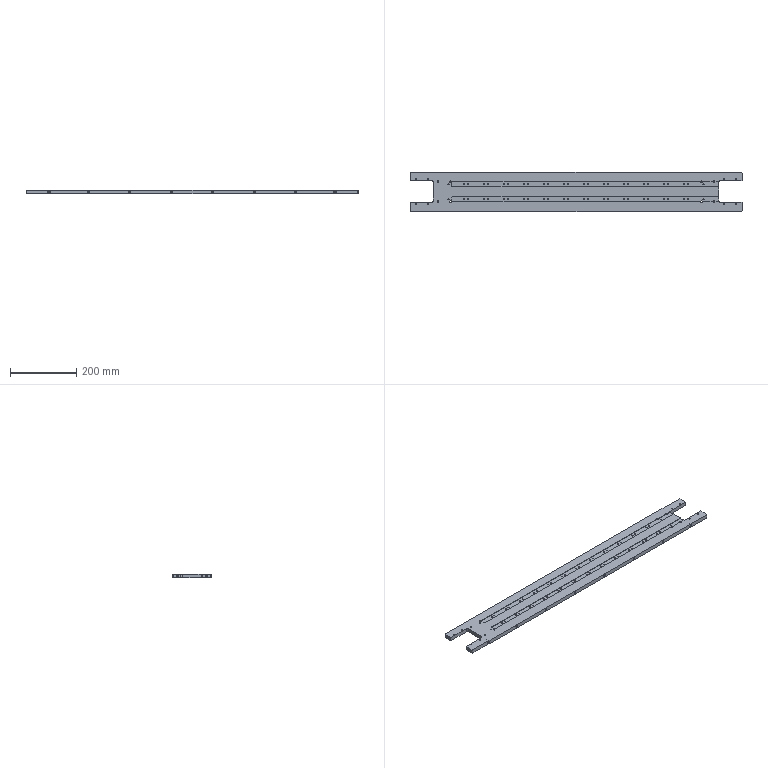Part | SolidWorks | features HoleWzd 11, ICE 3, MirrorPattern 3, Chamfer 2, Cut 2, Fillet 2, LPattern 2, MoveFace 2, Extrusion 1 | 1 solid | 238 faces | box 1000 x 118 x 12 mm | volume 1222730 mm3 | cylinder 172 | plane 42 | cone 24 | commonest cylinder face diameters 3.3 x120 5 x36 8 x16